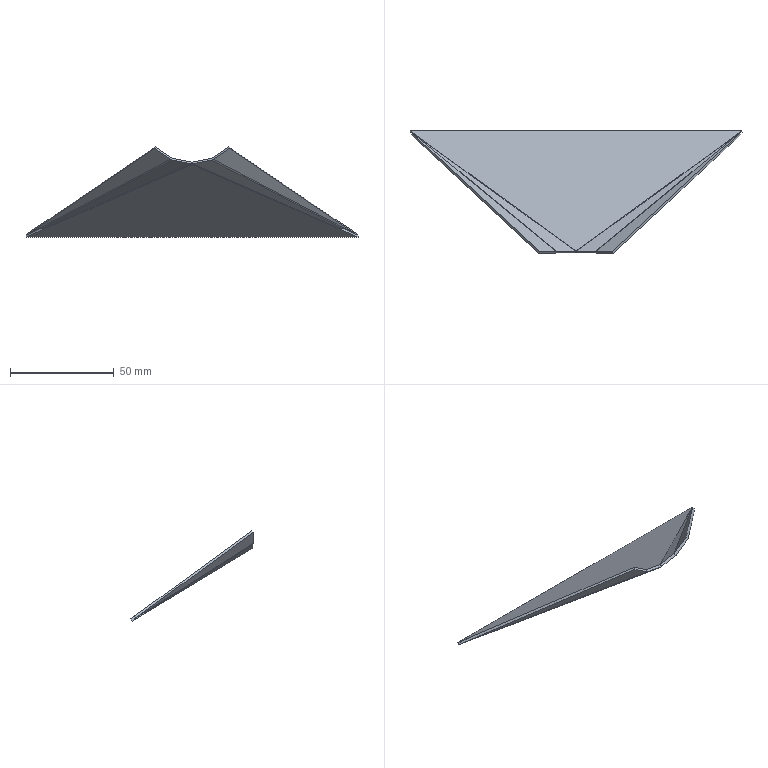Part | STEP file | JBJ-P-1003-010 | 1 solid | 42 faces | box 159.641 x 58.923 x 43.35 mm | volume 8515 mm3 | plane 32 | cylinder 8 | spline 2 | commonest cylinder face diameters 2 x4 4.4 x4
STEP:
#1=CARTESIAN_POINT('',(-7.275,-185.214,-25.075));
#2=VERTEX_POINT('',#1);
#3=CARTESIAN_POINT('',(-7.452,-185.997,-25.967));
#4=VERTEX_POINT('',#3);
#5=CARTESIAN_POINT('',(-7.275,-185.214,-25.075));
#6=DIRECTION('',(-0.1478,-0.6525,-0.7433));
#7=VECTOR('',#6,1000.);
#8=LINE('',#5,#7);
#9=EDGE_CURVE('',#2,#4,#8,.T.);
#10=ORIENTED_EDGE('',*,*,#9,.F.);
#11=CARTESIAN_POINT('',(-7.033,-185.39,-24.969));
#12=VERTEX_POINT('',#11);
#13=CARTESIAN_POINT('',(-74.854,-136.22,-54.641));
#14=DIRECTION('',(0.7632,-0.5533,0.3339));
#15=VECTOR('',#14,1000.);
#16=LINE('',#13,#15);
#17=EDGE_CURVE('',#2,#12,#16,.T.);
#18=ORIENTED_EDGE('',*,*,#17,.T.);
#19=CARTESIAN_POINT('',(-7.21,-186.173,-25.861));
#20=VERTEX_POINT('',#19);
#21=CARTESIAN_POINT('',(-7.033,-185.39,-24.969));
#22=DIRECTION('',(-0.1478,-0.6525,-0.7433));
#23=VECTOR('',#22,1000.);
#24=LINE('',#21,#23);
#25=EDGE_CURVE('',#12,#20,#24,.T.);
#26=ORIENTED_EDGE('',*,*,#25,.T.);
#27=CARTESIAN_POINT('',(-75.031,-137.003,-55.533));
#28=DIRECTION('',(0.7632,-0.5533,0.3339));
#29=VECTOR('',#28,1000.);
#30=LINE('',#27,#29);
#31=EDGE_CURVE('',#4,#20,#30,.T.);
#32=ORIENTED_EDGE('',*,*,#31,.F.);
#33=EDGE_LOOP('',(#10,#18,#26,#32));
#34=FACE_OUTER_BOUND('',#33,.T.);
#35=CARTESIAN_POINT('',(-74.854,-136.22,-54.641));
#36=DIRECTION('',(0.6291,0.5179,-0.5797));
#37=DIRECTION('',(0.7632,-0.5533,0.3339));
#38=AXIS2_PLACEMENT_3D('',#35,#36,#37);
#39=PLANE('',#38);
#40=ADVANCED_FACE('',(#34),#39,.T.);
#41=ORIENTED_EDGE('',*,*,#25,.F.);
#42=CARTESIAN_POINT('',(-16.241,-185.39,-23.137));
#43=VERTEX_POINT('',#42);
#44=CARTESIAN_POINT('',(-6.877,-185.39,-25.));
#45=DIRECTION('',(-0.9808,0.,0.1951));
#46=VECTOR('',#45,1000.);
#47=LINE('',#44,#46);
#48=EDGE_CURVE('',#12,#43,#47,.T.);
#49=ORIENTED_EDGE('',*,*,#48,.T.);
#50=CARTESIAN_POINT('',(-16.418,-186.173,-24.029));
#51=VERTEX_POINT('',#50);
#52=CARTESIAN_POINT('',(-16.241,-185.39,-23.137));
#53=DIRECTION('',(-0.1478,-0.6525,-0.7433));
#54=VECTOR('',#53,1000.);
#55=LINE('',#52,#54);
#56=EDGE_CURVE('',#43,#51,#55,.T.);
#57=ORIENTED_EDGE('',*,*,#56,.T.);
#58=CARTESIAN_POINT('',(-7.055,-186.173,-25.892));
#59=DIRECTION('',(-0.9808,0.,0.1951));
#60=VECTOR('',#59,1000.);
#61=LINE('',#58,#60);
#62=EDGE_CURVE('',#20,#51,#61,.T.);
#63=ORIENTED_EDGE('',*,*,#62,.F.);
#64=EDGE_LOOP('',(#41,#49,#57,#63));
#65=FACE_OUTER_BOUND('',#64,.T.);
#66=CARTESIAN_POINT('',(-6.877,-185.39,-25.));
#67=DIRECTION('',(0.1273,-0.7578,0.6399));
#68=DIRECTION('',(-0.9808,0.,0.1951));
#69=AXIS2_PLACEMENT_3D('',#66,#67,#68);
#70=PLANE('',#69);
#71=ADVANCED_FACE('',(#65),#70,.T.);
#72=ORIENTED_EDGE('',*,*,#56,.F.);
#73=CARTESIAN_POINT('',(-16.59,-185.39,-23.));
#74=VERTEX_POINT('',#73);
#75=CARTESIAN_POINT('',(-16.241,-185.39,-23.137));
#76=CARTESIAN_POINT('',(-16.376,-185.39,-23.111));
#77=CARTESIAN_POINT('',(-16.493,-185.39,-23.064));
#78=CARTESIAN_POINT('',(-16.59,-185.39,-23.));
#79=(BOUNDED_CURVE()B_SPLINE_CURVE(3,(#75,#76,#77,#78),.UNSPECIFIED.,.F.,.F.)B_SPLINE_CURVE_WITH_KNOTS((4,4),(5.652,5.972),.UNSPECIFIED.)CURVE()GEOMETRIC_REPRESENTATION_ITEM()RATIONAL_B_SPLINE_CURVE((1.,0.9915,0.9915,1.))REPRESENTATION_ITEM(''));
#80=EDGE_CURVE('',#43,#74,#79,.T.);
#81=ORIENTED_EDGE('',*,*,#80,.T.);
#82=CARTESIAN_POINT('',(-17.016,-186.313,-23.637));
#83=VERTEX_POINT('',#82);
#84=CARTESIAN_POINT('',(-16.59,-185.39,-23.));
#85=DIRECTION('',(-0.355,-0.7692,-0.5313));
#86=VECTOR('',#85,1000.);
#87=LINE('',#84,#86);
#88=EDGE_CURVE('',#74,#83,#87,.T.);
#89=ORIENTED_EDGE('',*,*,#88,.T.);
#90=CARTESIAN_POINT('',(-16.418,-186.173,-24.029));
#91=CARTESIAN_POINT('',(-16.641,-186.234,-23.931));
#92=CARTESIAN_POINT('',(-16.842,-186.281,-23.8));
#93=CARTESIAN_POINT('',(-17.016,-186.313,-23.637));
#94=(BOUNDED_CURVE()B_SPLINE_CURVE(3,(#90,#91,#92,#93),.UNSPECIFIED.,.F.,.T.)B_SPLINE_CURVE_WITH_KNOTS((4,4),(5.652,5.972),.UNSPECIFIED.)CURVE()GEOMETRIC_REPRESENTATION_ITEM()RATIONAL_B_SPLINE_CURVE((1.,0.9915,0.9915,1.))REPRESENTATION_ITEM(''));
#95=EDGE_CURVE('',#51,#83,#94,.T.);
#96=ORIENTED_EDGE('',*,*,#95,.F.);
#97=EDGE_LOOP('',(#72,#81,#89,#96));
#98=FACE_OUTER_BOUND('',#97,.T.);
#99=CARTESIAN_POINT('',(-17.43,-186.36,-23.095));
#100=CARTESIAN_POINT('',(-17.221,-186.036,-22.985));
#101=CARTESIAN_POINT('',(-17.013,-185.713,-22.876));
#102=CARTESIAN_POINT('',(-16.804,-185.39,-22.767));
#103=CARTESIAN_POINT('',(-19.472,-186.36,-19.197));
#104=CARTESIAN_POINT('',(-18.892,-186.036,-19.797));
#105=CARTESIAN_POINT('',(-18.312,-185.713,-20.396));
#106=CARTESIAN_POINT('',(-17.732,-185.39,-20.995));
#107=CARTESIAN_POINT('',(-15.213,-184.421,-16.966));
#108=CARTESIAN_POINT('',(-15.051,-184.744,-17.784));
#109=CARTESIAN_POINT('',(-14.888,-185.067,-18.602));
#110=CARTESIAN_POINT('',(-14.726,-185.39,-19.42));
#111=CARTESIAN_POINT('',(-13.171,-184.421,-20.863));
#112=CARTESIAN_POINT('',(-13.38,-184.744,-20.973));
#113=CARTESIAN_POINT('',(-13.589,-185.067,-21.082));
#114=CARTESIAN_POINT('',(-13.798,-185.39,-21.192));
#115=CARTESIAN_POINT('',(-11.129,-184.421,-24.761));
#116=CARTESIAN_POINT('',(-11.709,-184.744,-24.162));
#117=CARTESIAN_POINT('',(-12.289,-185.067,-23.562));
#118=CARTESIAN_POINT('',(-12.869,-185.39,-22.963));
#119=CARTESIAN_POINT('',(-15.388,-186.36,-26.992));
#120=CARTESIAN_POINT('',(-15.551,-186.036,-26.174));
#121=CARTESIAN_POINT('',(-15.713,-185.713,-25.356));
#122=CARTESIAN_POINT('',(-15.876,-185.39,-24.538));
#123=CARTESIAN_POINT('',(-17.43,-186.36,-23.095));
#124=CARTESIAN_POINT('',(-17.221,-186.036,-22.985));
#125=CARTESIAN_POINT('',(-17.013,-185.713,-22.876));
#126=CARTESIAN_POINT('',(-16.804,-185.39,-22.767));
#127=(BOUNDED_SURFACE()B_SPLINE_SURFACE(3,3,((#99,#100,#101,#102),(#103,#104,#105,#106),(#107,#108,#109,#110),(#111,#112,#113,#114),(#115,#116,#117,#118),(#119,#120,#121,#122),(#123,#124,#125,#126)),.UNSPECIFIED.,.T.,.F.,.F.)B_SPLINE_SURFACE_WITH_KNOTS((4,3,4),(4,4),(0.,0.5,1.),(0.,1.),.UNSPECIFIED.)GEOMETRIC_REPRESENTATION_ITEM()RATIONAL_B_SPLINE_SURFACE(((1.,1.,1.,1.),(0.3333,0.3333,0.3333,0.3333),(0.3333,0.3333,0.3333,0.3333),(1.,1.,1.,1.),(0.3333,0.3333,0.3333,0.3333),(0.3333,0.3333,0.3333,0.3333),(1.,1.,1.,1.)))REPRESENTATION_ITEM('')SURFACE());
#128=ADVANCED_FACE('',(#98),#127,.F.);
#129=ORIENTED_EDGE('',*,*,#88,.F.);
#130=CARTESIAN_POINT('',(-24.555,-185.39,-17.678));
#131=VERTEX_POINT('',#130);
#132=CARTESIAN_POINT('',(-16.444,-185.39,-23.097));
#133=DIRECTION('',(-0.8315,0.,0.5556));
#134=VECTOR('',#133,1000.);
#135=LINE('',#132,#134);
#136=EDGE_CURVE('',#74,#131,#135,.T.);
#137=ORIENTED_EDGE('',*,*,#136,.T.);
#138=CARTESIAN_POINT('',(-24.981,-186.313,-18.315));
#139=VERTEX_POINT('',#138);
#140=CARTESIAN_POINT('',(-24.555,-185.39,-17.678));
#141=DIRECTION('',(-0.355,-0.7692,-0.5313));
#142=VECTOR('',#141,1000.);
#143=LINE('',#140,#142);
#144=EDGE_CURVE('',#131,#139,#143,.T.);
#145=ORIENTED_EDGE('',*,*,#144,.T.);
#146=CARTESIAN_POINT('',(-16.87,-186.313,-23.735));
#147=DIRECTION('',(-0.8315,0.,0.5556));
#148=VECTOR('',#147,1000.);
#149=LINE('',#146,#148);
#150=EDGE_CURVE('',#83,#139,#149,.T.);
#151=ORIENTED_EDGE('',*,*,#150,.F.);
#152=EDGE_LOOP('',(#129,#137,#145,#151));
#153=FACE_OUTER_BOUND('',#152,.T.);
#154=CARTESIAN_POINT('',(-16.444,-185.39,-23.097));
#155=DIRECTION('',(0.4273,-0.639,0.6396));
#156=DIRECTION('',(-0.8315,0.,0.5556));
#157=AXIS2_PLACEMENT_3D('',#154,#155,#156);
#158=PLANE('',#157);
#159=ADVANCED_FACE('',(#153),#158,.T.);
#160=ORIENTED_EDGE('',*,*,#144,.F.);
#161=CARTESIAN_POINT('',(-85.759,-128.43,-59.241));
#162=VERTEX_POINT('',#161);
#163=CARTESIAN_POINT('',(-24.555,-185.39,-17.678));
#164=DIRECTION('',(-0.6555,0.61,-0.4451));
#165=VECTOR('',#164,1000.);
#166=LINE('',#163,#165);
#167=EDGE_CURVE('',#131,#162,#166,.T.);
#168=ORIENTED_EDGE('',*,*,#167,.T.);
#169=CARTESIAN_POINT('',(-86.185,-129.353,-59.879));
#170=VERTEX_POINT('',#169);
#171=CARTESIAN_POINT('',(-85.759,-128.43,-59.241));
#172=DIRECTION('',(-0.355,-0.7692,-0.5313));
#173=VECTOR('',#172,1000.);
#174=LINE('',#171,#173);
#175=EDGE_CURVE('',#162,#170,#174,.T.);
#176=ORIENTED_EDGE('',*,*,#175,.T.);
#177=CARTESIAN_POINT('',(-24.981,-186.313,-18.315));
#178=DIRECTION('',(-0.6555,0.61,-0.4451));
#179=VECTOR('',#178,1000.);
#180=LINE('',#177,#179);
#181=EDGE_CURVE('',#139,#170,#180,.T.);
#182=ORIENTED_EDGE('',*,*,#181,.F.);
#183=EDGE_LOOP('',(#160,#168,#176,#182));
#184=FACE_OUTER_BOUND('',#183,.T.);
#185=CARTESIAN_POINT('',(-24.555,-185.39,-17.678));
#186=DIRECTION('',(-0.6665,-0.1903,0.7208));
#187=DIRECTION('',(-0.6555,0.61,-0.4451));
#188=AXIS2_PLACEMENT_3D('',#185,#186,#187);
#189=PLANE('',#188);
#190=ADVANCED_FACE('',(#184),#189,.T.);
#191=ORIENTED_EDGE('',*,*,#175,.F.);
#192=CARTESIAN_POINT('',(-79.295,-133.754,-55.854));
#193=VERTEX_POINT('',#192);
#194=CARTESIAN_POINT('',(-80.106,-133.086,-56.279));
#195=DIRECTION('',(-0.7156,0.5893,-0.375));
#196=VECTOR('',#195,1000.);
#197=LINE('',#194,#196);
#198=EDGE_CURVE('',#193,#162,#197,.T.);
#199=ORIENTED_EDGE('',*,*,#198,.F.);
#200=CARTESIAN_POINT('',(-79.721,-134.677,-56.491));
#201=VERTEX_POINT('',#200);
#202=CARTESIAN_POINT('',(-79.295,-133.754,-55.854));
#203=DIRECTION('',(-0.355,-0.7692,-0.5313));
#204=VECTOR('',#203,1000.);
#205=LINE('',#202,#204);
#206=EDGE_CURVE('',#193,#201,#205,.T.);
#207=ORIENTED_EDGE('',*,*,#206,.T.);
#208=CARTESIAN_POINT('',(-80.532,-134.009,-56.917));
#209=DIRECTION('',(-0.7156,0.5893,-0.375));
#210=VECTOR('',#209,1000.);
#211=LINE('',#208,#210);
#212=EDGE_CURVE('',#201,#170,#211,.T.);
#213=ORIENTED_EDGE('',*,*,#212,.T.);
#214=EDGE_LOOP('',(#191,#199,#207,#213));
#215=FACE_OUTER_BOUND('',#214,.T.);
#216=CARTESIAN_POINT('',(-80.106,-133.086,-56.279));
#217=DIRECTION('',(-0.6015,-0.2471,0.7597));
#218=DIRECTION('',(-0.7156,0.5893,-0.375));
#219=AXIS2_PLACEMENT_3D('',#216,#217,#218);
#220=PLANE('',#219);
#221=ADVANCED_FACE('',(#215),#220,.F.);
#222=ORIENTED_EDGE('',*,*,#206,.F.);
#223=CARTESIAN_POINT('',(-79.087,-133.637,-56.066));
#224=VERTEX_POINT('',#223);
#225=CARTESIAN_POINT('',(-78.94,-132.985,-55.322));
#226=DIRECTION('',(0.7156,-0.5893,0.375));
#227=DIRECTION('',(0.6357,0.7719,0.));
#228=AXIS2_PLACEMENT_3D('',#225,#226,#227);
#229=CIRCLE('',#228,1.);
#230=EDGE_CURVE('',#193,#224,#229,.T.);
#231=ORIENTED_EDGE('',*,*,#230,.T.);
#232=CARTESIAN_POINT('',(-79.265,-134.42,-56.958));
#233=VERTEX_POINT('',#232);
#234=CARTESIAN_POINT('',(-79.087,-133.637,-56.066));
#235=DIRECTION('',(-0.1478,-0.6525,-0.7433));
#236=VECTOR('',#235,1000.);
#237=LINE('',#234,#236);
#238=EDGE_CURVE('',#224,#233,#237,.T.);
#239=ORIENTED_EDGE('',*,*,#238,.T.);
#240=CARTESIAN_POINT('',(-78.94,-132.985,-55.322));
#241=DIRECTION('',(0.7156,-0.5893,0.375));
#242=DIRECTION('',(-0.6357,-0.7719,0.));
#243=AXIS2_PLACEMENT_3D('',#240,#241,#242);
#244=CIRCLE('',#243,2.2);
#245=EDGE_CURVE('',#201,#233,#244,.T.);
#246=ORIENTED_EDGE('',*,*,#245,.F.);
#247=EDGE_LOOP('',(#222,#231,#239,#246));
#248=FACE_OUTER_BOUND('',#247,.T.);
#249=CARTESIAN_POINT('',(-78.94,-132.985,-55.322));
#250=DIRECTION('',(-0.7156,0.5893,-0.375));
#251=DIRECTION('',(-0.6357,-0.7719,0.));
#252=AXIS2_PLACEMENT_3D('',#249,#250,#251);
#253=PLANE('',#252);
#254=ADVANCED_FACE('',(#248),#253,.T.);
#255=ORIENTED_EDGE('',*,*,#238,.F.);
#256=CARTESIAN_POINT('',(-78.759,-133.388,-56.349));
#257=VERTEX_POINT('',#256);
#258=CARTESIAN_POINT('',(-22.262,-90.561,-105.181));
#259=DIRECTION('',(0.6563,0.4975,-0.5673));
#260=VECTOR('',#259,1000.);
#261=LINE('',#258,#260);
#262=EDGE_CURVE('',#224,#257,#261,.T.);
#263=ORIENTED_EDGE('',*,*,#262,.T.);
#264=CARTESIAN_POINT('',(-78.937,-134.171,-57.241));
#265=VERTEX_POINT('',#264);
#266=CARTESIAN_POINT('',(-78.759,-133.388,-56.349));
#267=DIRECTION('',(-0.1478,-0.6525,-0.7433));
#268=VECTOR('',#267,1000.);
#269=LINE('',#266,#268);
#270=EDGE_CURVE('',#257,#265,#269,.T.);
#271=ORIENTED_EDGE('',*,*,#270,.T.);
#272=CARTESIAN_POINT('',(-22.439,-91.344,-106.073));
#273=DIRECTION('',(0.6563,0.4975,-0.5673));
#274=VECTOR('',#273,1000.);
#275=LINE('',#272,#274);
#276=EDGE_CURVE('',#233,#265,#275,.T.);
#277=ORIENTED_EDGE('',*,*,#276,.F.);
#278=EDGE_LOOP('',(#255,#263,#271,#277));
#279=FACE_OUTER_BOUND('',#278,.T.);
#280=CARTESIAN_POINT('',(-22.262,-90.561,-105.181));
#281=DIRECTION('',(-0.7399,0.5717,-0.3546));
#282=DIRECTION('',(0.6563,0.4975,-0.5673));
#283=AXIS2_PLACEMENT_3D('',#280,#281,#282);
#284=PLANE('',#283);
#285=ADVANCED_FACE('',(#279),#284,.T.);
#286=ORIENTED_EDGE('',*,*,#270,.F.);
#287=CARTESIAN_POINT('',(-78.611,-133.253,-56.462));
#288=VERTEX_POINT('',#287);
#289=CARTESIAN_POINT('',(-78.611,-132.736,-55.606));
#290=DIRECTION('',(0.7632,-0.5533,0.3339));
#291=DIRECTION('',(-0.587,-0.8096,0.));
#292=AXIS2_PLACEMENT_3D('',#289,#290,#291);
#293=CIRCLE('',#292,1.);
#294=EDGE_CURVE('',#257,#288,#293,.T.);
#295=ORIENTED_EDGE('',*,*,#294,.T.);
#296=CARTESIAN_POINT('',(-78.611,-133.873,-57.49));
#297=VERTEX_POINT('',#296);
#298=CARTESIAN_POINT('',(-78.611,-133.253,-56.462));
#299=DIRECTION('',(0.,-0.5167,-0.8562));
#300=VECTOR('',#299,1000.);
#301=LINE('',#298,#300);
#302=EDGE_CURVE('',#288,#297,#301,.T.);
#303=ORIENTED_EDGE('',*,*,#302,.T.);
#304=CARTESIAN_POINT('',(-78.611,-132.736,-55.606));
#305=DIRECTION('',(0.7632,-0.5533,0.3339));
#306=DIRECTION('',(0.587,0.8096,0.));
#307=AXIS2_PLACEMENT_3D('',#304,#305,#306);
#308=CIRCLE('',#307,2.2);
#309=EDGE_CURVE('',#265,#297,#308,.T.);
#310=ORIENTED_EDGE('',*,*,#309,.F.);
#311=EDGE_LOOP('',(#286,#295,#303,#310));
#312=FACE_OUTER_BOUND('',#311,.T.);
#313=CARTESIAN_POINT('',(-78.611,-132.736,-55.606));
#314=DIRECTION('',(0.7632,-0.5533,0.3339));
#315=DIRECTION('',(0.587,0.8096,0.));
#316=AXIS2_PLACEMENT_3D('',#313,#314,#315);
#317=PLANE('',#316);
#318=ADVANCED_FACE('',(#312),#317,.F.);
#319=ORIENTED_EDGE('',*,*,#302,.F.);
#320=CARTESIAN_POINT('',(-86.698,-127.39,-60.));
#321=VERTEX_POINT('',#320);
#322=CARTESIAN_POINT('',(-74.706,-136.084,-54.754));
#323=DIRECTION('',(-0.7632,0.5533,-0.3339));
#324=VECTOR('',#323,1000.);
#325=LINE('',#322,#324);
#326=EDGE_CURVE('',#288,#321,#325,.T.);
#327=ORIENTED_EDGE('',*,*,#326,.T.);
#328=CARTESIAN_POINT('',(-86.698,-128.01,-61.027));
#329=VERTEX_POINT('',#328);
#330=CARTESIAN_POINT('',(-86.698,-127.39,-60.));
#331=DIRECTION('',(0.,-0.5167,-0.8562));
#332=VECTOR('',#331,1000.);
#333=LINE('',#330,#332);
#334=EDGE_CURVE('',#321,#329,#333,.T.);
#335=ORIENTED_EDGE('',*,*,#334,.T.);
#336=CARTESIAN_POINT('',(-74.706,-136.704,-55.781));
#337=DIRECTION('',(-0.7632,0.5533,-0.3339));
#338=VECTOR('',#337,1000.);
#339=LINE('',#336,#338);
#340=EDGE_CURVE('',#297,#329,#339,.T.);
#341=ORIENTED_EDGE('',*,*,#340,.F.);
#342=EDGE_LOOP('',(#319,#327,#335,#341));
#343=FACE_OUTER_BOUND('',#342,.T.);
#344=CARTESIAN_POINT('',(-74.706,-136.084,-54.754));
#345=DIRECTION('',(-0.6462,-0.6534,0.3943));
#346=DIRECTION('',(-0.7632,0.5533,-0.3339));
#347=AXIS2_PLACEMENT_3D('',#344,#345,#346);
#348=PLANE('',#347);
#349=ADVANCED_FACE('',(#343),#348,.T.);
#350=ORIENTED_EDGE('',*,*,#334,.F.);
#351=CARTESIAN_POINT('',(72.943,-127.39,-60.));
#352=VERTEX_POINT('',#351);
#353=CARTESIAN_POINT('',(-86.877,-127.39,-60.));
#354=DIRECTION('',(1.,0.,0.));
#355=VECTOR('',#354,1000.);
#356=LINE('',#353,#355);
#357=EDGE_CURVE('',#321,#352,#356,.T.);
#358=ORIENTED_EDGE('',*,*,#357,.T.);
#359=CARTESIAN_POINT('',(72.943,-128.01,-61.027));
#360=VERTEX_POINT('',#359);
#361=CARTESIAN_POINT('',(72.943,-127.39,-60.));
#362=DIRECTION('',(0.,-0.5167,-0.8562));
#363=VECTOR('',#362,1000.);
#364=LINE('',#361,#363);
#365=EDGE_CURVE('',#352,#360,#364,.T.);
#366=ORIENTED_EDGE('',*,*,#365,.T.);
#367=CARTESIAN_POINT('',(0.,-128.01,-61.027));
#368=DIRECTION('',(1.,0.,0.));
#369=VECTOR('',#368,1000.);
#370=LINE('',#367,#369);
#371=EDGE_CURVE('',#329,#360,#370,.T.);
#372=ORIENTED_EDGE('',*,*,#371,.F.);
#373=EDGE_LOOP('',(#350,#358,#366,#372));
#374=FACE_OUTER_BOUND('',#373,.T.);
#375=CARTESIAN_POINT('',(-86.877,-127.39,-60.));
#376=DIRECTION('',(0.,0.8562,-0.5167));
#377=DIRECTION('',(1.,0.,0.));
#378=AXIS2_PLACEMENT_3D('',#375,#376,#377);
#379=PLANE('',#378);
#380=ADVANCED_FACE('',(#374),#379,.T.);
#381=ORIENTED_EDGE('',*,*,#365,.F.);
#382=CARTESIAN_POINT('',(64.857,-133.253,-56.462));
#383=VERTEX_POINT('',#382);
#384=CARTESIAN_POINT('',(68.962,-130.276,-58.258));
#385=DIRECTION('',(0.7632,0.5533,-0.3339));
#386=VECTOR('',#385,1000.);
#387=LINE('',#384,#386);
#388=EDGE_CURVE('',#383,#352,#387,.T.);
#389=ORIENTED_EDGE('',*,*,#388,.F.);
#390=CARTESIAN_POINT('',(64.857,-133.873,-57.49));
#391=VERTEX_POINT('',#390);
#392=CARTESIAN_POINT('',(64.857,-133.253,-56.462));
#393=DIRECTION('',(0.,-0.5167,-0.8562));
#394=VECTOR('',#393,1000.);
#395=LINE('',#392,#394);
#396=EDGE_CURVE('',#383,#391,#395,.T.);
#397=ORIENTED_EDGE('',*,*,#396,.T.);
#398=CARTESIAN_POINT('',(68.962,-130.896,-59.286));
#399=DIRECTION('',(0.7632,0.5533,-0.3339));
#400=VECTOR('',#399,1000.);
#401=LINE('',#398,#400);
#402=EDGE_CURVE('',#391,#360,#401,.T.);
#403=ORIENTED_EDGE('',*,*,#402,.T.);
#404=EDGE_LOOP('',(#381,#389,#397,#403));
#405=FACE_OUTER_BOUND('',#404,.T.);
#406=CARTESIAN_POINT('',(68.962,-130.276,-58.258));
#407=DIRECTION('',(-0.6462,0.6534,-0.3943));
#408=DIRECTION('',(0.7632,0.5533,-0.3339));
#409=AXIS2_PLACEMENT_3D('',#406,#407,#408);
#410=PLANE('',#409);
#411=ADVANCED_FACE('',(#405),#410,.F.);
#412=ORIENTED_EDGE('',*,*,#396,.F.);
#413=CARTESIAN_POINT('',(65.005,-133.388,-56.349));
#414=VERTEX_POINT('',#413);
#415=CARTESIAN_POINT('',(64.857,-132.736,-55.606));
#416=DIRECTION('',(-0.7632,-0.5533,0.3339));
#417=DIRECTION('',(-0.587,0.8096,0.));
#418=AXIS2_PLACEMENT_3D('',#415,#416,#417);
#419=CIRCLE('',#418,1.);
#420=EDGE_CURVE('',#383,#414,#419,.T.);
#421=ORIENTED_EDGE('',*,*,#420,.T.);
#422=CARTESIAN_POINT('',(65.182,-134.171,-57.241));
#423=VERTEX_POINT('',#422);
#424=CARTESIAN_POINT('',(65.005,-133.388,-56.349));
#425=DIRECTION('',(0.1478,-0.6525,-0.7433));
#426=VECTOR('',#425,1000.);
#427=LINE('',#424,#426);
#428=EDGE_CURVE('',#414,#423,#427,.T.);
#429=ORIENTED_EDGE('',*,*,#428,.T.);
#430=CARTESIAN_POINT('',(64.857,-132.736,-55.606));
#431=DIRECTION('',(-0.7632,-0.5533,0.3339));
#432=DIRECTION('',(0.587,-0.8096,0.));
#433=AXIS2_PLACEMENT_3D('',#430,#431,#432);
#434=CIRCLE('',#433,2.2);
#435=EDGE_CURVE('',#391,#423,#434,.T.);
#436=ORIENTED_EDGE('',*,*,#435,.F.);
#437=EDGE_LOOP('',(#412,#421,#429,#436));
#438=FACE_OUTER_BOUND('',#437,.T.);
#439=CARTESIAN_POINT('',(64.857,-132.736,-55.606));
#440=DIRECTION('',(-0.7632,-0.5533,0.3339));
#441=DIRECTION('',(0.587,-0.8096,0.));
#442=AXIS2_PLACEMENT_3D('',#439,#440,#441);
#443=PLANE('',#442);
#444=ADVANCED_FACE('',(#438),#443,.F.);
#445=ORIENTED_EDGE('',*,*,#428,.F.);
#446=CARTESIAN_POINT('',(65.333,-133.637,-56.066));
#447=VERTEX_POINT('',#446);
#448=CARTESIAN_POINT('',(14.432,-95.052,-100.061));
#449=DIRECTION('',(-0.6563,0.4975,-0.5673));
#450=VECTOR('',#449,1000.);
#451=LINE('',#448,#450);
#452=EDGE_CURVE('',#447,#414,#451,.T.);
#453=ORIENTED_EDGE('',*,*,#452,.F.);
#454=CARTESIAN_POINT('',(65.51,-134.42,-56.958));
#455=VERTEX_POINT('',#454);
#456=CARTESIAN_POINT('',(65.333,-133.637,-56.066));
#457=DIRECTION('',(0.1478,-0.6525,-0.7433));
#458=VECTOR('',#457,1000.);
#459=LINE('',#456,#458);
#460=EDGE_CURVE('',#447,#455,#459,.T.);
#461=ORIENTED_EDGE('',*,*,#460,.T.);
#462=CARTESIAN_POINT('',(14.609,-95.835,-100.953));
#463=DIRECTION('',(-0.6563,0.4975,-0.5673));
#464=VECTOR('',#463,1000.);
#465=LINE('',#462,#464);
#466=EDGE_CURVE('',#455,#423,#465,.T.);
#467=ORIENTED_EDGE('',*,*,#466,.T.);
#468=EDGE_LOOP('',(#445,#453,#461,#467));
#469=FACE_OUTER_BOUND('',#468,.T.);
#470=CARTESIAN_POINT('',(14.432,-95.052,-100.061));
#471=DIRECTION('',(0.7399,0.5717,-0.3546));
#472=DIRECTION('',(-0.6563,0.4975,-0.5673));
#473=AXIS2_PLACEMENT_3D('',#470,#471,#472);
#474=PLANE('',#473);
#475=ADVANCED_FACE('',(#469),#474,.T.);
#476=ORIENTED_EDGE('',*,*,#460,.F.);
#477=CARTESIAN_POINT('',(65.54,-133.754,-55.854));
#478=VERTEX_POINT('',#477);
#479=CARTESIAN_POINT('',(65.185,-132.985,-55.322));
#480=DIRECTION('',(-0.7156,-0.5893,0.375));
#481=DIRECTION('',(-0.6357,0.7719,0.));
#482=AXIS2_PLACEMENT_3D('',#479,#480,#481);
#483=CIRCLE('',#482,1.);
#484=EDGE_CURVE('',#447,#478,#483,.T.);
#485=ORIENTED_EDGE('',*,*,#484,.T.);
#486=CARTESIAN_POINT('',(65.966,-134.677,-56.491));
#487=VERTEX_POINT('',#486);
#488=CARTESIAN_POINT('',(65.54,-133.754,-55.854));
#489=DIRECTION('',(0.355,-0.7692,-0.5313));
#490=VECTOR('',#489,1000.);
#491=LINE('',#488,#490);
#492=EDGE_CURVE('',#478,#487,#491,.T.);
#493=ORIENTED_EDGE('',*,*,#492,.T.);
#494=CARTESIAN_POINT('',(65.185,-132.985,-55.322));
#495=DIRECTION('',(-0.7156,-0.5893,0.375));
#496=DIRECTION('',(-0.6357,0.7719,0.));
#497=AXIS2_PLACEMENT_3D('',#494,#495,#496);
#498=CIRCLE('',#497,2.2);
#499=EDGE_CURVE('',#455,#487,#498,.T.);
#500=ORIENTED_EDGE('',*,*,#499,.F.);
#501=EDGE_LOOP('',(#476,#485,#493,#500));
#502=FACE_OUTER_BOUND('',#501,.T.);
#503=CARTESIAN_POINT('',(65.185,-132.985,-55.322));
#504=DIRECTION('',(-0.7156,-0.5893,0.375));
#505=DIRECTION('',(0.6357,-0.7719,0.));
#506=AXIS2_PLACEMENT_3D('',#503,#504,#505);
#507=PLANE('',#506);
#508=ADVANCED_FACE('',(#502),#507,.F.);
#509=ORIENTED_EDGE('',*,*,#492,.F.);
#510=CARTESIAN_POINT('',(72.005,-128.43,-59.241));
#511=VERTEX_POINT('',#510);
#512=CARTESIAN_POINT('',(73.396,-127.285,-59.97));
#513=DIRECTION('',(-0.7156,-0.5893,0.375));
#514=VECTOR('',#513,1000.);
#515=LINE('',#512,#514);
#516=EDGE_CURVE('',#511,#478,#515,.T.);
#517=ORIENTED_EDGE('',*,*,#516,.F.);
#518=CARTESIAN_POINT('',(72.431,-129.353,-59.879));
#519=VERTEX_POINT('',#518);
#520=CARTESIAN_POINT('',(72.005,-128.43,-59.241));
#521=DIRECTION('',(0.355,-0.7692,-0.5313));
#522=VECTOR('',#521,1000.);
#523=LINE('',#520,#522);
#524=EDGE_CURVE('',#511,#519,#523,.T.);
#525=ORIENTED_EDGE('',*,*,#524,.T.);
#526=CARTESIAN_POINT('',(73.822,-128.208,-60.607));
#527=DIRECTION('',(-0.7156,-0.5893,0.375));
#528=VECTOR('',#527,1000.);
#529=LINE('',#526,#528);
#530=EDGE_CURVE('',#519,#487,#529,.T.);
#531=ORIENTED_EDGE('',*,*,#530,.T.);
#532=EDGE_LOOP('',(#509,#517,#525,#531));
#533=FACE_OUTER_BOUND('',#532,.T.);
#534=CARTESIAN_POINT('',(73.396,-127.285,-59.97));
#535=DIRECTION('',(-0.6015,0.2471,-0.7597));
#536=DIRECTION('',(-0.7156,-0.5893,0.375));
#537=AXIS2_PLACEMENT_3D('',#534,#535,#536);
#538=PLANE('',#537);
#539=ADVANCED_FACE('',(#533),#538,.T.);
#540=ORIENTED_EDGE('',*,*,#524,.F.);
#541=CARTESIAN_POINT('',(10.801,-185.39,-17.678));
#542=VERTEX_POINT('',#541);
#543=CARTESIAN_POINT('',(73.123,-127.39,-60.));
#544=DIRECTION('',(-0.6555,-0.61,0.4451));
#545=VECTOR('',#544,1000.);
#546=LINE('',#543,#545);
#547=EDGE_CURVE('',#511,#542,#546,.T.);
#548=ORIENTED_EDGE('',*,*,#547,.T.);
#549=CARTESIAN_POINT('',(11.227,-186.313,-18.315));
#550=VERTEX_POINT('',#549);
#551=CARTESIAN_POINT('',(10.801,-185.39,-17.678));
#552=DIRECTION('',(0.355,-0.7692,-0.5313));
#553=VECTOR('',#552,1000.);
#554=LINE('',#551,#553);
#555=EDGE_CURVE('',#542,#550,#554,.T.);
#556=ORIENTED_EDGE('',*,*,#555,.T.);
#557=CARTESIAN_POINT('',(73.549,-128.313,-60.638));
#558=DIRECTION('',(-0.6555,-0.61,0.4451));
#559=VECTOR('',#558,1000.);
#560=LINE('',#557,#559);
#561=EDGE_CURVE('',#519,#550,#560,.T.);
#562=ORIENTED_EDGE('',*,*,#561,.F.);
#563=EDGE_LOOP('',(#540,#548,#556,#562));
#564=FACE_OUTER_BOUND('',#563,.T.);
#565=CARTESIAN_POINT('',(73.123,-127.39,-60.));
#566=DIRECTION('',(-0.6665,0.1903,-0.7208));
#567=DIRECTION('',(-0.6555,-0.61,0.4451));
#568=AXIS2_PLACEMENT_3D('',#565,#566,#567);
#569=PLANE('',#568);
#570=ADVANCED_FACE('',(#564),#569,.F.);
#571=ORIENTED_EDGE('',*,*,#555,.F.);
#572=CARTESIAN_POINT('',(2.835,-185.39,-23.));
#573=VERTEX_POINT('',#572);
#574=CARTESIAN_POINT('',(10.801,-185.39,-17.678));
#575=DIRECTION('',(-0.8315,0.,-0.5556));
#576=VECTOR('',#575,1000.);
#577=LINE('',#574,#576);
#578=EDGE_CURVE('',#542,#573,#577,.T.);
#579=ORIENTED_EDGE('',*,*,#578,.T.);
#580=CARTESIAN_POINT('',(3.261,-186.313,-23.637));
#581=VERTEX_POINT('',#580);
#582=CARTESIAN_POINT('',(2.835,-185.39,-23.));
#583=DIRECTION('',(0.355,-0.7692,-0.5313));
#584=VECTOR('',#583,1000.);
#585=LINE('',#582,#584);
#586=EDGE_CURVE('',#573,#581,#585,.T.);
#587=ORIENTED_EDGE('',*,*,#586,.T.);
#588=CARTESIAN_POINT('',(11.227,-186.313,-18.315));
#589=DIRECTION('',(-0.8315,0.,-0.5556));
#590=VECTOR('',#589,1000.);
#591=LINE('',#588,#590);
#592=EDGE_CURVE('',#550,#581,#591,.T.);
#593=ORIENTED_EDGE('',*,*,#592,.F.);
#594=EDGE_LOOP('',(#571,#579,#587,#593));
#595=FACE_OUTER_BOUND('',#594,.T.);
#596=CARTESIAN_POINT('',(10.801,-185.39,-17.678));
#597=DIRECTION('',(0.4273,0.639,-0.6396));
#598=DIRECTION('',(-0.8315,0.,-0.5556));
#599=AXIS2_PLACEMENT_3D('',#596,#597,#598);
#600=PLANE('',#599);
#601=ADVANCED_FACE('',(#595),#600,.F.);
#602=ORIENTED_EDGE('',*,*,#586,.F.);
#603=CARTESIAN_POINT('',(2.486,-185.39,-23.137));
#604=VERTEX_POINT('',#603);
#605=CARTESIAN_POINT('',(2.835,-185.39,-23.));
#606=CARTESIAN_POINT('',(2.739,-185.39,-23.064));
#607=CARTESIAN_POINT('',(2.622,-185.39,-23.111));
#608=CARTESIAN_POINT('',(2.486,-185.39,-23.137));
#609=(BOUNDED_CURVE()B_SPLINE_CURVE(3,(#605,#606,#607,#608),.UNSPECIFIED.,.F.,.F.)B_SPLINE_CURVE_WITH_KNOTS((4,4),(0.3109,0.6308),.UNSPECIFIED.)CURVE()GEOMETRIC_REPRESENTATION_ITEM()RATIONAL_B_SPLINE_CURVE((1.,0.9915,0.9915,1.))REPRESENTATION_ITEM(''));
#610=EDGE_CURVE('',#573,#604,#609,.T.);
#611=ORIENTED_EDGE('',*,*,#610,.T.);
#612=CARTESIAN_POINT('',(2.664,-186.173,-24.029));
#613=VERTEX_POINT('',#612);
#614=CARTESIAN_POINT('',(2.486,-185.39,-23.137));
#615=DIRECTION('',(0.1478,-0.6525,-0.7433));
#616=VECTOR('',#615,1000.);
#617=LINE('',#614,#616);
#618=EDGE_CURVE('',#604,#613,#617,.T.);
#619=ORIENTED_EDGE('',*,*,#618,.T.);
#620=CARTESIAN_POINT('',(3.261,-186.313,-23.637));
#621=CARTESIAN_POINT('',(3.088,-186.281,-23.8));
#622=CARTESIAN_POINT('',(2.887,-186.234,-23.931));
#623=CARTESIAN_POINT('',(2.664,-186.173,-24.029));
#624=(BOUNDED_CURVE()B_SPLINE_CURVE(3,(#620,#621,#622,#623),.UNSPECIFIED.,.F.,.T.)B_SPLINE_CURVE_WITH_KNOTS((4,4),(0.3109,0.6308),.UNSPECIFIED.)CURVE()GEOMETRIC_REPRESENTATION_ITEM()RATIONAL_B_SPLINE_CURVE((1.,0.9915,0.9915,1.))REPRESENTATION_ITEM(''));
#625=EDGE_CURVE('',#581,#613,#624,.T.);
#626=ORIENTED_EDGE('',*,*,#625,.F.);
#627=EDGE_LOOP('',(#602,#611,#619,#626));
#628=FACE_OUTER_BOUND('',#627,.T.);
#629=CARTESIAN_POINT('',(3.676,-186.36,-23.095));
#630=CARTESIAN_POINT('',(3.467,-186.036,-22.985));
#631=CARTESIAN_POINT('',(3.258,-185.713,-22.876));
#632=CARTESIAN_POINT('',(3.049,-185.39,-22.767));
#633=CARTESIAN_POINT('',(1.634,-186.36,-26.992));
#634=CARTESIAN_POINT('',(1.796,-186.036,-26.174));
#635=CARTESIAN_POINT('',(1.959,-185.713,-25.356));
#636=CARTESIAN_POINT('',(2.121,-185.39,-24.538));
#637=CARTESIAN_POINT('',(-2.625,-184.421,-24.761));
#638=CARTESIAN_POINT('',(-2.045,-184.744,-24.162));
#639=CARTESIAN_POINT('',(-1.465,-185.067,-23.562));
#640=CARTESIAN_POINT('',(-0.885,-185.39,-22.963));
#641=CARTESIAN_POINT('',(-0.5832,-184.421,-20.863));
#642=CARTESIAN_POINT('',(-0.3744,-184.744,-20.973));
#643=CARTESIAN_POINT('',(-0.1656,-185.067,-21.082));
#644=CARTESIAN_POINT('',(0.04319,-185.39,-21.192));
#645=CARTESIAN_POINT('',(1.459,-184.421,-16.966));
#646=CARTESIAN_POINT('',(1.296,-184.744,-17.784));
#647=CARTESIAN_POINT('',(1.134,-185.067,-18.602));
#648=CARTESIAN_POINT('',(0.9714,-185.39,-19.42));
#649=CARTESIAN_POINT('',(5.718,-186.36,-19.197));
#650=CARTESIAN_POINT('',(5.138,-186.036,-19.797));
#651=CARTESIAN_POINT('',(4.558,-185.713,-20.396));
#652=CARTESIAN_POINT('',(3.978,-185.39,-20.995));
#653=CARTESIAN_POINT('',(3.676,-186.36,-23.095));
#654=CARTESIAN_POINT('',(3.467,-186.036,-22.985));
#655=CARTESIAN_POINT('',(3.258,-185.713,-22.876));
#656=CARTESIAN_POINT('',(3.049,-185.39,-22.767));
#657=(BOUNDED_SURFACE()B_SPLINE_SURFACE(3,3,((#629,#630,#631,#632),(#633,#634,#635,#636),(#637,#638,#639,#640),(#641,#642,#643,#644),(#645,#646,#647,#648),(#649,#650,#651,#652),(#653,#654,#655,#656)),.UNSPECIFIED.,.T.,.F.,.F.)B_SPLINE_SURFACE_WITH_KNOTS((4,3,4),(4,4),(0.,0.5,1.),(0.,1.),.UNSPECIFIED.)GEOMETRIC_REPRESENTATION_ITEM()RATIONAL_B_SPLINE_SURFACE(((1.,1.,1.,1.),(0.3333,0.3333,0.3333,0.3333),(0.3333,0.3333,0.3333,0.3333),(1.,1.,1.,1.),(0.3333,0.3333,0.3333,0.3333),(0.3333,0.3333,0.3333,0.3333),(1.,1.,1.,1.)))REPRESENTATION_ITEM('')SURFACE());
#658=ADVANCED_FACE('',(#628),#657,.F.);
#659=ORIENTED_EDGE('',*,*,#618,.F.);
#660=CARTESIAN_POINT('',(-6.721,-185.39,-24.969));
#661=VERTEX_POINT('',#660);
#662=CARTESIAN_POINT('',(2.69,-185.39,-23.097));
#663=DIRECTION('',(-0.9808,0.,-0.1951));
#664=VECTOR('',#663,1000.);
#665=LINE('',#662,#664);
#666=EDGE_CURVE('',#604,#661,#665,.T.);
#667=ORIENTED_EDGE('',*,*,#666,.T.);
#668=CARTESIAN_POINT('',(-6.544,-186.173,-25.861));
#669=VERTEX_POINT('',#668);
#670=CARTESIAN_POINT('',(-6.721,-185.39,-24.969));
#671=DIRECTION('',(0.1478,-0.6525,-0.7433));
#672=VECTOR('',#671,1000.);
#673=LINE('',#670,#672);
#674=EDGE_CURVE('',#661,#669,#673,.T.);
#675=ORIENTED_EDGE('',*,*,#674,.T.);
#676=CARTESIAN_POINT('',(2.867,-186.173,-23.989));
#677=DIRECTION('',(-0.9808,0.,-0.1951));
#678=VECTOR('',#677,1000.);
#679=LINE('',#676,#678);
#680=EDGE_CURVE('',#613,#669,#679,.T.);
#681=ORIENTED_EDGE('',*,*,#680,.F.);
#682=EDGE_LOOP('',(#659,#667,#675,#681));
#683=FACE_OUTER_BOUND('',#682,.T.);
#684=CARTESIAN_POINT('',(2.69,-185.39,-23.097));
#685=DIRECTION('',(0.1273,0.7578,-0.6399));
#686=DIRECTION('',(-0.9808,0.,-0.1951));
#687=AXIS2_PLACEMENT_3D('',#684,#685,#686);
#688=PLANE('',#687);
#689=ADVANCED_FACE('',(#683),#688,.F.);
#690=ORIENTED_EDGE('',*,*,#674,.F.);
#691=CARTESIAN_POINT('',(-6.479,-185.214,-25.075));
#692=VERTEX_POINT('',#691);
#693=CARTESIAN_POINT('',(69.11,-130.412,-58.145));
#694=DIRECTION('',(0.7632,0.5533,-0.3339));
#695=VECTOR('',#694,1000.);
#696=LINE('',#693,#695);
#697=EDGE_CURVE('',#661,#692,#696,.T.);
#698=ORIENTED_EDGE('',*,*,#697,.T.);
#699=CARTESIAN_POINT('',(-6.302,-185.997,-25.967));
#700=VERTEX_POINT('',#699);
#701=CARTESIAN_POINT('',(-6.479,-185.214,-25.075));
#702=DIRECTION('',(0.1478,-0.6525,-0.7433));
#703=VECTOR('',#702,1000.);
#704=LINE('',#701,#703);
#705=EDGE_CURVE('',#692,#700,#704,.T.);
#706=ORIENTED_EDGE('',*,*,#705,.T.);
#707=CARTESIAN_POINT('',(69.288,-131.195,-59.037));
#708=DIRECTION('',(0.7632,0.5533,-0.3339));
#709=VECTOR('',#708,1000.);
#710=LINE('',#707,#709);
#711=EDGE_CURVE('',#669,#700,#710,.T.);
#712=ORIENTED_EDGE('',*,*,#711,.F.);
#713=EDGE_LOOP('',(#690,#698,#706,#712));
#714=FACE_OUTER_BOUND('',#713,.T.);
#715=CARTESIAN_POINT('',(69.11,-130.412,-58.145));
#716=DIRECTION('',(0.6291,-0.5179,0.5797));
#717=DIRECTION('',(0.7632,0.5533,-0.3339));
#718=AXIS2_PLACEMENT_3D('',#715,#716,#717);
#719=PLANE('',#718);
#720=ADVANCED_FACE('',(#714),#719,.F.);
#721=ORIENTED_EDGE('',*,*,#705,.F.);
#722=CARTESIAN_POINT('',(-6.627,-185.079,-25.188));
#723=VERTEX_POINT('',#722);
#724=CARTESIAN_POINT('',(-6.627,-184.562,-24.332));
#725=DIRECTION('',(0.7632,0.5533,-0.3339));
#726=DIRECTION('',(-0.587,0.8096,0.));
#727=AXIS2_PLACEMENT_3D('',#724,#725,#726);
#728=CIRCLE('',#727,1.);
#729=EDGE_CURVE('',#692,#723,#728,.T.);
#730=ORIENTED_EDGE('',*,*,#729,.T.);
#731=CARTESIAN_POINT('',(-6.627,-185.699,-26.215));
#732=VERTEX_POINT('',#731);
#733=CARTESIAN_POINT('',(-6.627,-185.079,-25.188));
#734=DIRECTION('',(0.,-0.5167,-0.8562));
#735=VECTOR('',#734,1000.);
#736=LINE('',#733,#735);
#737=EDGE_CURVE('',#723,#732,#736,.T.);
#738=ORIENTED_EDGE('',*,*,#737,.T.);
#739=CARTESIAN_POINT('',(-6.627,-184.562,-24.332));
#740=DIRECTION('',(0.7632,0.5533,-0.3339));
#741=DIRECTION('',(0.587,-0.8096,0.));
#742=AXIS2_PLACEMENT_3D('',#739,#740,#741);
#743=CIRCLE('',#742,2.2);
#744=EDGE_CURVE('',#700,#732,#743,.T.);
#745=ORIENTED_EDGE('',*,*,#744,.F.);
#746=EDGE_LOOP('',(#721,#730,#738,#745));
#747=FACE_OUTER_BOUND('',#746,.T.);
#748=CARTESIAN_POINT('',(-6.627,-184.562,-24.332));
#749=DIRECTION('',(-0.7632,-0.5533,0.3339));
#750=DIRECTION('',(0.587,-0.8096,0.));
#751=AXIS2_PLACEMENT_3D('',#748,#749,#750);
#752=PLANE('',#751);
#753=ADVANCED_FACE('',(#747),#752,.T.);
#754=ORIENTED_EDGE('',*,*,#737,.F.);
#755=CARTESIAN_POINT('',(-7.127,-185.079,-25.188));
#756=VERTEX_POINT('',#755);
#757=CARTESIAN_POINT('',(0.,-185.079,-25.188));
#758=DIRECTION('',(1.,0.,0.));
#759=VECTOR('',#758,1000.);
#760=LINE('',#757,#759);
#761=EDGE_CURVE('',#756,#723,#760,.T.);
#762=ORIENTED_EDGE('',*,*,#761,.F.);
#763=CARTESIAN_POINT('',(-7.127,-185.699,-26.215));
#764=VERTEX_POINT('',#763);
#765=CARTESIAN_POINT('',(-7.127,-185.079,-25.188));
#766=DIRECTION('',(0.,-0.5167,-0.8562));
#767=VECTOR('',#766,1000.);
#768=LINE('',#765,#767);
#769=EDGE_CURVE('',#756,#764,#768,.T.);
#770=ORIENTED_EDGE('',*,*,#769,.T.);
#771=CARTESIAN_POINT('',(0.,-185.699,-26.215));
#772=DIRECTION('',(1.,0.,0.));
#773=VECTOR('',#772,1000.);
#774=LINE('',#771,#773);
#775=EDGE_CURVE('',#764,#732,#774,.T.);
#776=ORIENTED_EDGE('',*,*,#775,.T.);
#777=EDGE_LOOP('',(#754,#762,#770,#776));
#778=FACE_OUTER_BOUND('',#777,.T.);
#779=CARTESIAN_POINT('',(0.,-185.079,-25.188));
#780=DIRECTION('',(0.,0.8562,-0.5167));
#781=DIRECTION('',(1.,0.,0.));
#782=AXIS2_PLACEMENT_3D('',#779,#780,#781);
#783=PLANE('',#782);
#784=ADVANCED_FACE('',(#778),#783,.F.);
#785=CARTESIAN_POINT('',(-7.127,-184.562,-24.332));
#786=DIRECTION('',(-0.7632,0.5533,-0.3339));
#787=DIRECTION('',(-0.587,-0.8096,0.));
#788=AXIS2_PLACEMENT_3D('',#785,#786,#787);
#789=CIRCLE('',#788,1.);
#790=EDGE_CURVE('',#756,#2,#789,.T.);
#791=ORIENTED_EDGE('',*,*,#790,.T.);
#792=ORIENTED_EDGE('',*,*,#9,.T.);
#793=CARTESIAN_POINT('',(-7.127,-184.562,-24.332));
#794=DIRECTION('',(-0.7632,0.5533,-0.3339));
#795=DIRECTION('',(0.587,0.8096,0.));
#796=AXIS2_PLACEMENT_3D('',#793,#794,#795);
#797=CIRCLE('',#796,2.2);
#798=EDGE_CURVE('',#764,#4,#797,.T.);
#799=ORIENTED_EDGE('',*,*,#798,.F.);
#800=ORIENTED_EDGE('',*,*,#769,.F.);
#801=EDGE_LOOP('',(#791,#792,#799,#800));
#802=FACE_OUTER_BOUND('',#801,.T.);
#803=CARTESIAN_POINT('',(-7.127,-184.562,-24.332));
#804=DIRECTION('',(0.7632,-0.5533,0.3339));
#805=DIRECTION('',(0.587,0.8096,0.));
#806=AXIS2_PLACEMENT_3D('',#803,#804,#805);
#807=PLANE('',#806);
#808=ADVANCED_FACE('',(#802),#807,.T.);
#809=ORIENTED_EDGE('',*,*,#775,.F.);
#810=CARTESIAN_POINT('',(-74.706,-136.704,-55.781));
#811=DIRECTION('',(-0.7632,0.5533,-0.3339));
#812=VECTOR('',#811,1000.);
#813=LINE('',#810,#812);
#814=EDGE_CURVE('',#764,#297,#813,.T.);
#815=ORIENTED_EDGE('',*,*,#814,.T.);
#816=ORIENTED_EDGE('',*,*,#340,.T.);
#817=ORIENTED_EDGE('',*,*,#371,.T.);
#818=ORIENTED_EDGE('',*,*,#402,.F.);
#819=CARTESIAN_POINT('',(68.962,-130.896,-59.286));
#820=DIRECTION('',(-0.7632,-0.5533,0.3339));
#821=VECTOR('',#820,1000.);
#822=LINE('',#819,#821);
#823=EDGE_CURVE('',#391,#732,#822,.T.);
#824=ORIENTED_EDGE('',*,*,#823,.T.);
#825=EDGE_LOOP('',(#809,#815,#816,#817,#818,#824));
#826=FACE_OUTER_BOUND('',#825,.T.);
#827=CARTESIAN_POINT('',(0.,-61.168,-101.363));
#828=DIRECTION('',(0.,-0.5167,-0.8562));
#829=DIRECTION('',(0.,0.8562,-0.5167));
#830=AXIS2_PLACEMENT_3D('',#827,#828,#829);
#831=PLANE('',#830);
#832=ADVANCED_FACE('',(#826),#831,.T.);
#833=ORIENTED_EDGE('',*,*,#62,.T.);
#834=CARTESIAN_POINT('',(-80.076,-133.752,-57.383));
#835=DIRECTION('',(-0.7156,0.5893,-0.375));
#836=VECTOR('',#835,1000.);
#837=LINE('',#834,#836);
#838=EDGE_CURVE('',#51,#233,#837,.T.);
#839=ORIENTED_EDGE('',*,*,#838,.T.);
#840=ORIENTED_EDGE('',*,*,#276,.T.);
#841=CARTESIAN_POINT('',(-75.031,-137.003,-55.533));
#842=DIRECTION('',(0.7632,-0.5533,0.3339));
#843=VECTOR('',#842,1000.);
#844=LINE('',#841,#843);
#845=EDGE_CURVE('',#265,#4,#844,.T.);
#846=ORIENTED_EDGE('',*,*,#845,.T.);
#847=ORIENTED_EDGE('',*,*,#31,.T.);
#848=EDGE_LOOP('',(#833,#839,#840,#846,#847));
#849=FACE_OUTER_BOUND('',#848,.T.);
#850=CARTESIAN_POINT('',(-20.958,-92.489,-105.363));
#851=DIRECTION('',(-0.1478,-0.6525,-0.7433));
#852=DIRECTION('',(0.,0.7515,-0.6597));
#853=AXIS2_PLACEMENT_3D('',#850,#851,#852);
#854=PLANE('',#853);
#855=ADVANCED_FACE('',(#849),#854,.T.);
#856=ORIENTED_EDGE('',*,*,#592,.T.);
#857=CARTESIAN_POINT('',(73.822,-128.208,-60.607));
#858=DIRECTION('',(0.7156,0.5893,-0.375));
#859=VECTOR('',#858,1000.);
#860=LINE('',#857,#859);
#861=EDGE_CURVE('',#581,#487,#860,.T.);
#862=ORIENTED_EDGE('',*,*,#861,.T.);
#863=ORIENTED_EDGE('',*,*,#530,.F.);
#864=ORIENTED_EDGE('',*,*,#561,.T.);
#865=EDGE_LOOP('',(#856,#862,#863,#864));
#866=FACE_OUTER_BOUND('',#865,.T.);
#867=CARTESIAN_POINT('',(55.748,-120.783,-83.433));
#868=DIRECTION('',(-0.355,0.7692,0.5313));
#869=DIRECTION('',(0.,-0.5684,0.8228));
#870=AXIS2_PLACEMENT_3D('',#867,#868,#869);
#871=PLANE('',#870);
#872=ADVANCED_FACE('',(#866),#871,.F.);
#873=ORIENTED_EDGE('',*,*,#466,.F.);
#874=CARTESIAN_POINT('',(73.366,-127.951,-61.073));
#875=DIRECTION('',(-0.7156,-0.5893,0.375));
#876=VECTOR('',#875,1000.);
#877=LINE('',#874,#876);
#878=EDGE_CURVE('',#455,#613,#877,.T.);
#879=ORIENTED_EDGE('',*,*,#878,.T.);
#880=ORIENTED_EDGE('',*,*,#680,.T.);
#881=ORIENTED_EDGE('',*,*,#711,.T.);
#882=CARTESIAN_POINT('',(69.288,-131.195,-59.037));
#883=DIRECTION('',(0.7632,0.5533,-0.3339));
#884=VECTOR('',#883,1000.);
#885=LINE('',#882,#884);
#886=EDGE_CURVE('',#700,#423,#885,.T.);
#887=ORIENTED_EDGE('',*,*,#886,.T.);
#888=EDGE_LOOP('',(#873,#879,#880,#881,#887));
#889=FACE_OUTER_BOUND('',#888,.T.);
#890=CARTESIAN_POINT('',(20.657,-91.162,-103.852));
#891=DIRECTION('',(-0.1478,0.6525,0.7433));
#892=DIRECTION('',(0.,-0.7515,0.6597));
#893=AXIS2_PLACEMENT_3D('',#890,#891,#892);
#894=PLANE('',#893);
#895=ADVANCED_FACE('',(#889),#894,.F.);
#896=ORIENTED_EDGE('',*,*,#212,.F.);
#897=CARTESIAN_POINT('',(-80.532,-134.009,-56.917));
#898=DIRECTION('',(0.7156,-0.5893,0.375));
#899=VECTOR('',#898,1000.);
#900=LINE('',#897,#899);
#901=EDGE_CURVE('',#201,#83,#900,.T.);
#902=ORIENTED_EDGE('',*,*,#901,.T.);
#903=ORIENTED_EDGE('',*,*,#150,.T.);
#904=ORIENTED_EDGE('',*,*,#181,.T.);
#905=EDGE_LOOP('',(#896,#902,#903,#904));
#906=FACE_OUTER_BOUND('',#905,.T.);
#907=CARTESIAN_POINT('',(-57.482,-124.539,-86.027));
#908=DIRECTION('',(-0.355,-0.7692,-0.5313));
#909=DIRECTION('',(0.,0.5684,-0.8228));
#910=AXIS2_PLACEMENT_3D('',#907,#908,#909);
#911=PLANE('',#910);
#912=ADVANCED_FACE('',(#906),#911,.T.);
#913=ORIENTED_EDGE('',*,*,#744,.T.);
#914=ORIENTED_EDGE('',*,*,#823,.F.);
#915=ORIENTED_EDGE('',*,*,#435,.T.);
#916=ORIENTED_EDGE('',*,*,#886,.F.);
#917=EDGE_LOOP('',(#913,#914,#915,#916));
#918=FACE_OUTER_BOUND('',#917,.T.);
#919=CARTESIAN_POINT('',(68.962,-129.76,-57.402));
#920=DIRECTION('',(-0.7632,-0.5533,0.3339));
#921=DIRECTION('',(0.587,-0.8096,0.));
#922=AXIS2_PLACEMENT_3D('',#919,#920,#921);
#923=CYLINDRICAL_SURFACE('',#922,2.2);
#924=ADVANCED_FACE('',(#918),#923,.T.);
#925=ORIENTED_EDGE('',*,*,#625,.T.);
#926=ORIENTED_EDGE('',*,*,#878,.F.);
#927=ORIENTED_EDGE('',*,*,#499,.T.);
#928=ORIENTED_EDGE('',*,*,#861,.F.);
#929=EDGE_LOOP('',(#925,#926,#927,#928));
#930=FACE_OUTER_BOUND('',#929,.T.);
#931=CARTESIAN_POINT('',(73.041,-126.516,-59.438));
#932=DIRECTION('',(0.7156,0.5893,-0.375));
#933=DIRECTION('',(-0.6357,0.7719,0.));
#934=AXIS2_PLACEMENT_3D('',#931,#932,#933);
#935=CYLINDRICAL_SURFACE('',#934,2.2);
#936=ADVANCED_FACE('',(#930),#935,.T.);
#937=ORIENTED_EDGE('',*,*,#309,.T.);
#938=ORIENTED_EDGE('',*,*,#814,.F.);
#939=ORIENTED_EDGE('',*,*,#798,.T.);
#940=ORIENTED_EDGE('',*,*,#845,.F.);
#941=EDGE_LOOP('',(#937,#938,#939,#940));
#942=FACE_OUTER_BOUND('',#941,.T.);
#943=CARTESIAN_POINT('',(-74.706,-135.567,-53.897));
#944=DIRECTION('',(0.7632,-0.5533,0.3339));
#945=DIRECTION('',(0.587,0.8096,0.));
#946=AXIS2_PLACEMENT_3D('',#943,#944,#945);
#947=CYLINDRICAL_SURFACE('',#946,2.2);
#948=ADVANCED_FACE('',(#942),#947,.T.);
#949=ORIENTED_EDGE('',*,*,#95,.T.);
#950=ORIENTED_EDGE('',*,*,#901,.F.);
#951=ORIENTED_EDGE('',*,*,#245,.T.);
#952=ORIENTED_EDGE('',*,*,#838,.F.);
#953=EDGE_LOOP('',(#949,#950,#951,#952));
#954=FACE_OUTER_BOUND('',#953,.T.);
#955=CARTESIAN_POINT('',(-79.751,-132.316,-55.748));
#956=DIRECTION('',(-0.7156,0.5893,-0.375));
#957=DIRECTION('',(-0.6357,-0.7719,0.));
#958=AXIS2_PLACEMENT_3D('',#955,#956,#957);
#959=CYLINDRICAL_SURFACE('',#958,2.2);
#960=ADVANCED_FACE('',(#954),#959,.T.);
#961=ORIENTED_EDGE('',*,*,#761,.T.);
#962=CARTESIAN_POINT('',(-6.627,-185.079,-25.188));
#963=DIRECTION('',(-0.7632,-0.5533,0.3339));
#964=VECTOR('',#963,1000.);
#965=LINE('',#962,#964);
#966=EDGE_CURVE('',#383,#723,#965,.T.);
#967=ORIENTED_EDGE('',*,*,#966,.F.);
#968=ORIENTED_EDGE('',*,*,#388,.T.);
#969=ORIENTED_EDGE('',*,*,#357,.F.);
#970=ORIENTED_EDGE('',*,*,#326,.F.);
#971=CARTESIAN_POINT('',(-74.706,-136.084,-54.754));
#972=DIRECTION('',(-0.7632,0.5533,-0.3339));
#973=VECTOR('',#972,1000.);
#974=LINE('',#971,#973);
#975=EDGE_CURVE('',#756,#288,#974,.T.);
#976=ORIENTED_EDGE('',*,*,#975,.F.);
#977=EDGE_LOOP('',(#961,#967,#968,#969,#970,#976));
#978=FACE_OUTER_BOUND('',#977,.T.);
#979=CARTESIAN_POINT('',(0.,-60.548,-100.336));
#980=DIRECTION('',(0.,-0.5167,-0.8562));
#981=DIRECTION('',(0.,0.8562,-0.5167));
#982=AXIS2_PLACEMENT_3D('',#979,#980,#981);
#983=PLANE('',#982);
#984=ADVANCED_FACE('',(#978),#983,.F.);
#985=ORIENTED_EDGE('',*,*,#48,.F.);
#986=ORIENTED_EDGE('',*,*,#17,.F.);
#987=CARTESIAN_POINT('',(-74.854,-136.22,-54.641));
#988=DIRECTION('',(0.7632,-0.5533,0.3339));
#989=VECTOR('',#988,1000.);
#990=LINE('',#987,#989);
#991=EDGE_CURVE('',#257,#2,#990,.T.);
#992=ORIENTED_EDGE('',*,*,#991,.F.);
#993=ORIENTED_EDGE('',*,*,#262,.F.);
#994=CARTESIAN_POINT('',(-79.899,-132.969,-56.491));
#995=DIRECTION('',(-0.7156,0.5893,-0.375));
#996=VECTOR('',#995,1000.);
#997=LINE('',#994,#996);
#998=EDGE_CURVE('',#43,#224,#997,.T.);
#999=ORIENTED_EDGE('',*,*,#998,.F.);
#1000=EDGE_LOOP('',(#985,#986,#992,#993,#999));
#1001=FACE_OUTER_BOUND('',#1000,.T.);
#1002=CARTESIAN_POINT('',(-20.781,-91.706,-104.471));
#1003=DIRECTION('',(-0.1478,-0.6525,-0.7433));
#1004=DIRECTION('',(0.,0.7515,-0.6597));
#1005=AXIS2_PLACEMENT_3D('',#1002,#1003,#1004);
#1006=PLANE('',#1005);
#1007=ADVANCED_FACE('',(#1001),#1006,.F.);
#1008=ORIENTED_EDGE('',*,*,#578,.F.);
#1009=ORIENTED_EDGE('',*,*,#547,.F.);
#1010=ORIENTED_EDGE('',*,*,#516,.T.);
#1011=CARTESIAN_POINT('',(73.396,-127.285,-59.97));
#1012=DIRECTION('',(0.7156,0.5893,-0.375));
#1013=VECTOR('',#1012,1000.);
#1014=LINE('',#1011,#1013);
#1015=EDGE_CURVE('',#573,#478,#1014,.T.);
#1016=ORIENTED_EDGE('',*,*,#1015,.F.);
#1017=EDGE_LOOP('',(#1008,#1009,#1010,#1016));
#1018=FACE_OUTER_BOUND('',#1017,.T.);
#1019=CARTESIAN_POINT('',(55.322,-119.86,-82.795));
#1020=DIRECTION('',(-0.355,0.7692,0.5313));
#1021=DIRECTION('',(0.,-0.5684,0.8228));
#1022=AXIS2_PLACEMENT_3D('',#1019,#1020,#1021);
#1023=PLANE('',#1022);
#1024=ADVANCED_FACE('',(#1018),#1023,.T.);
#1025=ORIENTED_EDGE('',*,*,#452,.T.);
#1026=CARTESIAN_POINT('',(65.005,-133.388,-56.349));
#1027=DIRECTION('',(0.7632,0.5533,-0.3339));
#1028=VECTOR('',#1027,1000.);
#1029=LINE('',#1026,#1028);
#1030=EDGE_CURVE('',#692,#414,#1029,.T.);
#1031=ORIENTED_EDGE('',*,*,#1030,.F.);
#1032=ORIENTED_EDGE('',*,*,#697,.F.);
#1033=ORIENTED_EDGE('',*,*,#666,.F.);
#1034=CARTESIAN_POINT('',(73.189,-127.168,-60.182));
#1035=DIRECTION('',(-0.7156,-0.5893,0.375));
#1036=VECTOR('',#1035,1000.);
#1037=LINE('',#1034,#1036);
#1038=EDGE_CURVE('',#447,#604,#1037,.T.);
#1039=ORIENTED_EDGE('',*,*,#1038,.F.);
#1040=EDGE_LOOP('',(#1025,#1031,#1032,#1033,#1039));
#1041=FACE_OUTER_BOUND('',#1040,.T.);
#1042=CARTESIAN_POINT('',(20.48,-90.379,-102.96));
#1043=DIRECTION('',(-0.1478,0.6525,0.7433));
#1044=DIRECTION('',(0.,-0.7515,0.6597));
#1045=AXIS2_PLACEMENT_3D('',#1042,#1043,#1044);
#1046=PLANE('',#1045);
#1047=ADVANCED_FACE('',(#1041),#1046,.T.);
#1048=ORIENTED_EDGE('',*,*,#198,.T.);
#1049=ORIENTED_EDGE('',*,*,#167,.F.);
#1050=ORIENTED_EDGE('',*,*,#136,.F.);
#1051=CARTESIAN_POINT('',(-80.106,-133.086,-56.279));
#1052=DIRECTION('',(0.7156,-0.5893,0.375));
#1053=VECTOR('',#1052,1000.);
#1054=LINE('',#1051,#1053);
#1055=EDGE_CURVE('',#193,#74,#1054,.T.);
#1056=ORIENTED_EDGE('',*,*,#1055,.F.);
#1057=EDGE_LOOP('',(#1048,#1049,#1050,#1056));
#1058=FACE_OUTER_BOUND('',#1057,.T.);
#1059=CARTESIAN_POINT('',(-57.056,-123.616,-85.39));
#1060=DIRECTION('',(-0.355,-0.7692,-0.5313));
#1061=DIRECTION('',(0.,0.5684,-0.8228));
#1062=AXIS2_PLACEMENT_3D('',#1059,#1060,#1061);
#1063=PLANE('',#1062);
#1064=ADVANCED_FACE('',(#1058),#1063,.F.);
#1065=ORIENTED_EDGE('',*,*,#729,.F.);
#1066=ORIENTED_EDGE('',*,*,#1030,.T.);
#1067=ORIENTED_EDGE('',*,*,#420,.F.);
#1068=ORIENTED_EDGE('',*,*,#966,.T.);
#1069=EDGE_LOOP('',(#1065,#1066,#1067,#1068));
#1070=FACE_OUTER_BOUND('',#1069,.T.);
#1071=CARTESIAN_POINT('',(68.962,-129.76,-57.402));
#1072=DIRECTION('',(-0.7632,-0.5533,0.3339));
#1073=DIRECTION('',(0.587,-0.8096,0.));
#1074=AXIS2_PLACEMENT_3D('',#1071,#1072,#1073);
#1075=CYLINDRICAL_SURFACE('',#1074,1.);
#1076=ADVANCED_FACE('',(#1070),#1075,.F.);
#1077=ORIENTED_EDGE('',*,*,#610,.F.);
#1078=ORIENTED_EDGE('',*,*,#1015,.T.);
#1079=ORIENTED_EDGE('',*,*,#484,.F.);
#1080=ORIENTED_EDGE('',*,*,#1038,.T.);
#1081=EDGE_LOOP('',(#1077,#1078,#1079,#1080));
#1082=FACE_OUTER_BOUND('',#1081,.T.);
#1083=CARTESIAN_POINT('',(73.041,-126.516,-59.438));
#1084=DIRECTION('',(0.7156,0.5893,-0.375));
#1085=DIRECTION('',(-0.6357,0.7719,0.));
#1086=AXIS2_PLACEMENT_3D('',#1083,#1084,#1085);
#1087=CYLINDRICAL_SURFACE('',#1086,1.);
#1088=ADVANCED_FACE('',(#1082),#1087,.F.);
#1089=ORIENTED_EDGE('',*,*,#294,.F.);
#1090=ORIENTED_EDGE('',*,*,#991,.T.);
#1091=ORIENTED_EDGE('',*,*,#790,.F.);
#1092=ORIENTED_EDGE('',*,*,#975,.T.);
#1093=EDGE_LOOP('',(#1089,#1090,#1091,#1092));
#1094=FACE_OUTER_BOUND('',#1093,.T.);
#1095=CARTESIAN_POINT('',(-74.706,-135.567,-53.897));
#1096=DIRECTION('',(0.7632,-0.5533,0.3339));
#1097=DIRECTION('',(0.587,0.8096,0.));
#1098=AXIS2_PLACEMENT_3D('',#1095,#1096,#1097);
#1099=CYLINDRICAL_SURFACE('',#1098,1.);
#1100=ADVANCED_FACE('',(#1094),#1099,.F.);
#1101=ORIENTED_EDGE('',*,*,#80,.F.);
#1102=ORIENTED_EDGE('',*,*,#998,.T.);
#1103=ORIENTED_EDGE('',*,*,#230,.F.);
#1104=ORIENTED_EDGE('',*,*,#1055,.T.);
#1105=EDGE_LOOP('',(#1101,#1102,#1103,#1104));
#1106=FACE_OUTER_BOUND('',#1105,.T.);
#1107=CARTESIAN_POINT('',(-79.751,-132.316,-55.748));
#1108=DIRECTION('',(-0.7156,0.5893,-0.375));
#1109=DIRECTION('',(-0.6357,-0.7719,0.));
#1110=AXIS2_PLACEMENT_3D('',#1107,#1108,#1109);
#1111=CYLINDRICAL_SURFACE('',#1110,1.);
#1112=ADVANCED_FACE('',(#1106),#1111,.F.);
#1113=CLOSED_SHELL('',(#40,#71,#128,#159,#190,#221,#254,#285,#318,#349,#380,#411,#444,#475,#508,#539,#570,#601,#658,#689,#720,#753,#784,#808,#832,#855,#872,#895,#912,#924,#936,#948,#960,#984,#1007,#1024,#1047,#1064,#1076,#1088,#1100,#1112));
#1114=MANIFOLD_SOLID_BREP('',#1113);
#1115=CARTESIAN_POINT('',(0.,0.,0.));
#1116=DIRECTION('',(0.,0.,1.));
#1117=DIRECTION('',(1.,0.,0.));
#1118=AXIS2_PLACEMENT_3D('',#1115,#1116,#1117);
#1119=(LENGTH_UNIT()NAMED_UNIT(*)SI_UNIT(.MILLI.,.METRE.));
#1120=UNCERTAINTY_MEASURE_WITH_UNIT(LENGTH_MEASURE(0.00001),#1119,'','');
#1121=(NAMED_UNIT(*)PLANE_ANGLE_UNIT()SI_UNIT($,.RADIAN.));
#1122=(NAMED_UNIT(*)SI_UNIT($,.STERADIAN.)SOLID_ANGLE_UNIT());
#1123=(GEOMETRIC_REPRESENTATION_CONTEXT(3)GLOBAL_UNCERTAINTY_ASSIGNED_CONTEXT((#1120))GLOBAL_UNIT_ASSIGNED_CONTEXT((#1119,#1121,#1122))REPRESENTATION_CONTEXT('',''));
#1124=ADVANCED_BREP_SHAPE_REPRESENTATION('',(#1114,#1118),#1123);